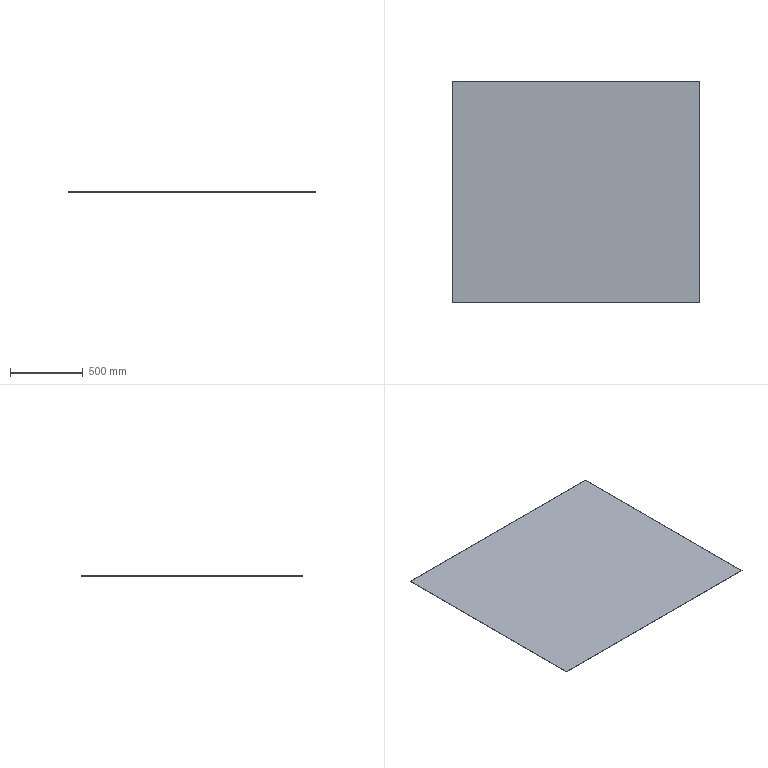Part | STEP file | Pad plate | 1 solid | 6 faces | box 1700 x 1520 x 2 mm | volume 5168000 mm3 | plane 6
STEP:
#1=CARTESIAN_POINT('',(0.,-320.,2.));
#2=VERTEX_POINT('',#1);
#3=CARTESIAN_POINT('',(0.,1200.,2.));
#4=VERTEX_POINT('',#3);
#5=CARTESIAN_POINT('',(0.,0.,2.));
#6=DIRECTION('',(0.,1.,0.));
#7=VECTOR('',#6,1000.);
#8=LINE('',#5,#7);
#9=EDGE_CURVE('',#2,#4,#8,.T.);
#10=ORIENTED_EDGE('',*,*,#9,.T.);
#11=CARTESIAN_POINT('',(-1700.,1200.,2.));
#12=VERTEX_POINT('',#11);
#13=CARTESIAN_POINT('',(0.,1200.,2.));
#14=DIRECTION('',(-1.,0.,0.));
#15=VECTOR('',#14,1000.);
#16=LINE('',#13,#15);
#17=EDGE_CURVE('',#4,#12,#16,.T.);
#18=ORIENTED_EDGE('',*,*,#17,.T.);
#19=CARTESIAN_POINT('',(-1700.,-320.,2.));
#20=VERTEX_POINT('',#19);
#21=CARTESIAN_POINT('',(-1700.,0.,2.));
#22=DIRECTION('',(0.,-1.,0.));
#23=VECTOR('',#22,1000.);
#24=LINE('',#21,#23);
#25=EDGE_CURVE('',#12,#20,#24,.T.);
#26=ORIENTED_EDGE('',*,*,#25,.T.);
#27=CARTESIAN_POINT('',(0.,-320.,2.));
#28=DIRECTION('',(1.,0.,0.));
#29=VECTOR('',#28,1000.);
#30=LINE('',#27,#29);
#31=EDGE_CURVE('',#20,#2,#30,.T.);
#32=ORIENTED_EDGE('',*,*,#31,.T.);
#33=EDGE_LOOP('',(#10,#18,#26,#32));
#34=FACE_OUTER_BOUND('',#33,.T.);
#35=CARTESIAN_POINT('',(0.,0.,2.));
#36=DIRECTION('',(0.,0.,1.));
#37=DIRECTION('',(1.,0.,0.));
#38=AXIS2_PLACEMENT_3D('',#35,#36,#37);
#39=PLANE('',#38);
#40=ADVANCED_FACE('',(#34),#39,.T.);
#41=CARTESIAN_POINT('',(-1700.,1200.,0.));
#42=VERTEX_POINT('',#41);
#43=CARTESIAN_POINT('',(-1700.,1200.,2.));
#44=DIRECTION('',(0.,0.,-1.));
#45=VECTOR('',#44,1000.);
#46=LINE('',#43,#45);
#47=EDGE_CURVE('',#12,#42,#46,.T.);
#48=ORIENTED_EDGE('',*,*,#47,.F.);
#49=ORIENTED_EDGE('',*,*,#17,.F.);
#50=CARTESIAN_POINT('',(0.,1200.,0.));
#51=VERTEX_POINT('',#50);
#52=CARTESIAN_POINT('',(0.,1200.,2.));
#53=DIRECTION('',(0.,0.,1.));
#54=VECTOR('',#53,1000.);
#55=LINE('',#52,#54);
#56=EDGE_CURVE('',#51,#4,#55,.T.);
#57=ORIENTED_EDGE('',*,*,#56,.F.);
#58=CARTESIAN_POINT('',(-1700.,1200.,0.));
#59=DIRECTION('',(1.,0.,0.));
#60=VECTOR('',#59,1000.);
#61=LINE('',#58,#60);
#62=EDGE_CURVE('',#42,#51,#61,.T.);
#63=ORIENTED_EDGE('',*,*,#62,.F.);
#64=EDGE_LOOP('',(#48,#49,#57,#63));
#65=FACE_OUTER_BOUND('',#64,.T.);
#66=CARTESIAN_POINT('',(-1700.,1200.,2.));
#67=DIRECTION('',(0.,-1.,0.));
#68=DIRECTION('',(0.,0.,-1.));
#69=AXIS2_PLACEMENT_3D('',#66,#67,#68);
#70=PLANE('',#69);
#71=ADVANCED_FACE('',(#65),#70,.F.);
#72=ORIENTED_EDGE('',*,*,#56,.T.);
#73=ORIENTED_EDGE('',*,*,#9,.F.);
#74=CARTESIAN_POINT('',(0.,-320.,0.));
#75=VERTEX_POINT('',#74);
#76=CARTESIAN_POINT('',(0.,-320.,0.));
#77=DIRECTION('',(0.,0.,-1.));
#78=VECTOR('',#77,1000.);
#79=LINE('',#76,#78);
#80=EDGE_CURVE('',#2,#75,#79,.T.);
#81=ORIENTED_EDGE('',*,*,#80,.T.);
#82=CARTESIAN_POINT('',(0.,1200.,0.));
#83=DIRECTION('',(0.,-1.,0.));
#84=VECTOR('',#83,1000.);
#85=LINE('',#82,#84);
#86=EDGE_CURVE('',#51,#75,#85,.T.);
#87=ORIENTED_EDGE('',*,*,#86,.F.);
#88=EDGE_LOOP('',(#72,#73,#81,#87));
#89=FACE_OUTER_BOUND('',#88,.T.);
#90=CARTESIAN_POINT('',(0.,1200.,2.));
#91=DIRECTION('',(-1.,0.,0.));
#92=DIRECTION('',(0.,-1.,0.));
#93=AXIS2_PLACEMENT_3D('',#90,#91,#92);
#94=PLANE('',#93);
#95=ADVANCED_FACE('',(#89),#94,.F.);
#96=CARTESIAN_POINT('',(-1700.,-320.,0.));
#97=VERTEX_POINT('',#96);
#98=CARTESIAN_POINT('',(-1700.,1200.,0.));
#99=DIRECTION('',(0.,1.,0.));
#100=VECTOR('',#99,1000.);
#101=LINE('',#98,#100);
#102=EDGE_CURVE('',#97,#42,#101,.T.);
#103=ORIENTED_EDGE('',*,*,#102,.F.);
#104=CARTESIAN_POINT('',(-1700.,-320.,2.));
#105=DIRECTION('',(0.,0.,1.));
#106=VECTOR('',#105,1000.);
#107=LINE('',#104,#106);
#108=EDGE_CURVE('',#97,#20,#107,.T.);
#109=ORIENTED_EDGE('',*,*,#108,.T.);
#110=ORIENTED_EDGE('',*,*,#25,.F.);
#111=ORIENTED_EDGE('',*,*,#47,.T.);
#112=EDGE_LOOP('',(#103,#109,#110,#111));
#113=FACE_OUTER_BOUND('',#112,.T.);
#114=CARTESIAN_POINT('',(-1700.,1200.,2.));
#115=DIRECTION('',(1.,0.,0.));
#116=DIRECTION('',(0.,1.,0.));
#117=AXIS2_PLACEMENT_3D('',#114,#115,#116);
#118=PLANE('',#117);
#119=ADVANCED_FACE('',(#113),#118,.F.);
#120=ORIENTED_EDGE('',*,*,#62,.T.);
#121=ORIENTED_EDGE('',*,*,#86,.T.);
#122=CARTESIAN_POINT('',(-1700.,-320.,0.));
#123=DIRECTION('',(-1.,0.,0.));
#124=VECTOR('',#123,1000.);
#125=LINE('',#122,#124);
#126=EDGE_CURVE('',#75,#97,#125,.T.);
#127=ORIENTED_EDGE('',*,*,#126,.T.);
#128=ORIENTED_EDGE('',*,*,#102,.T.);
#129=EDGE_LOOP('',(#120,#121,#127,#128));
#130=FACE_OUTER_BOUND('',#129,.T.);
#131=CARTESIAN_POINT('',(0.,0.,0.));
#132=DIRECTION('',(0.,0.,1.));
#133=DIRECTION('',(1.,0.,0.));
#134=AXIS2_PLACEMENT_3D('',#131,#132,#133);
#135=PLANE('',#134);
#136=ADVANCED_FACE('',(#130),#135,.F.);
#137=ORIENTED_EDGE('',*,*,#80,.F.);
#138=ORIENTED_EDGE('',*,*,#31,.F.);
#139=ORIENTED_EDGE('',*,*,#108,.F.);
#140=ORIENTED_EDGE('',*,*,#126,.F.);
#141=EDGE_LOOP('',(#137,#138,#139,#140));
#142=FACE_OUTER_BOUND('',#141,.T.);
#143=CARTESIAN_POINT('',(-1680.,-320.,56.));
#144=DIRECTION('',(0.,1.,0.));
#145=DIRECTION('',(0.,0.,-1.));
#146=AXIS2_PLACEMENT_3D('',#143,#144,#145);
#147=PLANE('',#146);
#148=ADVANCED_FACE('',(#142),#147,.F.);
#149=CLOSED_SHELL('',(#40,#71,#95,#119,#136,#148));
#150=MANIFOLD_SOLID_BREP('',#149);
#151=CARTESIAN_POINT('',(0.,0.,0.));
#152=DIRECTION('',(0.,0.,1.));
#153=DIRECTION('',(1.,0.,0.));
#154=AXIS2_PLACEMENT_3D('',#151,#152,#153);
#155=(LENGTH_UNIT()NAMED_UNIT(*)SI_UNIT(.MILLI.,.METRE.));
#156=UNCERTAINTY_MEASURE_WITH_UNIT(LENGTH_MEASURE(0.00001),#155,'','');
#157=(NAMED_UNIT(*)PLANE_ANGLE_UNIT()SI_UNIT($,.RADIAN.));
#158=(NAMED_UNIT(*)SI_UNIT($,.STERADIAN.)SOLID_ANGLE_UNIT());
#159=(GEOMETRIC_REPRESENTATION_CONTEXT(3)GLOBAL_UNCERTAINTY_ASSIGNED_CONTEXT((#156))GLOBAL_UNIT_ASSIGNED_CONTEXT((#155,#157,#158))REPRESENTATION_CONTEXT('',''));
#160=ADVANCED_BREP_SHAPE_REPRESENTATION('',(#150,#154),#159);